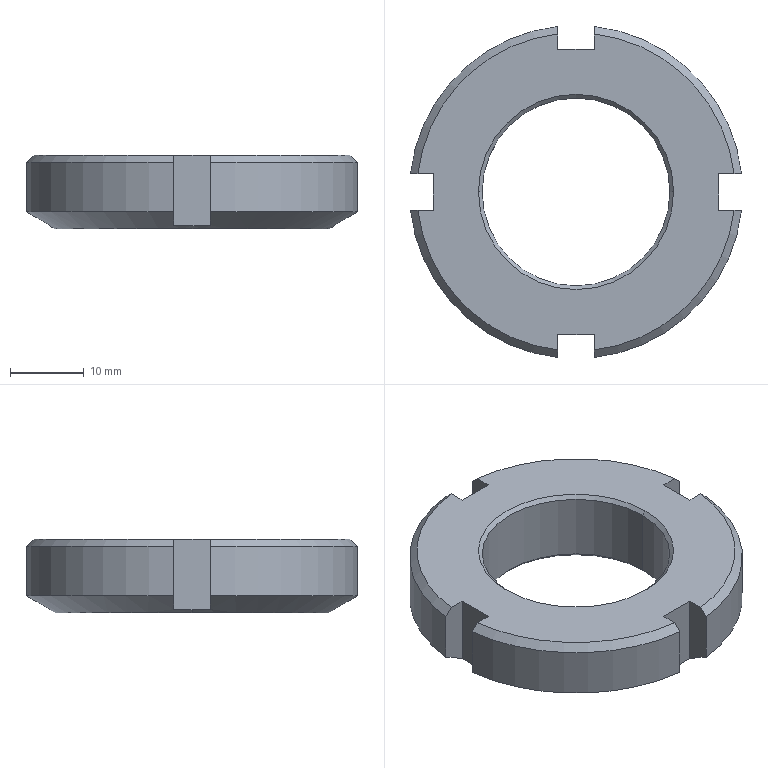Part | SolidWorks | features Chamfer 3, CirPattern 1, Cut 1, Extrusion 1 | 1 solid | 30 faces | box 44.721 x 44.721 x 10 mm | volume 9603 mm3 | plane 14 | cone 10 | cylinder 6 | commonest cylinder face diameters 45 x4 25.376 x2
STEP:
#1=CARTESIAN_POINT('',(-12.688,0.,9.5));
#2=VERTEX_POINT('',#1);
#3=CARTESIAN_POINT('',(12.688,0.,9.5));
#4=VERTEX_POINT('',#3);
#5=CARTESIAN_POINT('',(0.,0.,9.5));
#6=DIRECTION('',(0.,0.,1.));
#7=DIRECTION('',(1.,0.,0.));
#8=AXIS2_PLACEMENT_3D('',#5,#6,#7);
#9=CIRCLE('',#8,12.688);
#10=EDGE_CURVE('',#2,#4,#9,.T.);
#11=ORIENTED_EDGE('',*,*,#10,.F.);
#12=CARTESIAN_POINT('',(-13.188,0.,10.));
#13=VERTEX_POINT('',#12);
#14=CARTESIAN_POINT('',(-12.688,0.,9.5));
#15=DIRECTION('',(-0.7071,0.,0.7071));
#16=VECTOR('',#15,1000.);
#17=LINE('',#14,#16);
#18=EDGE_CURVE('',#2,#13,#17,.T.);
#19=ORIENTED_EDGE('',*,*,#18,.T.);
#20=CARTESIAN_POINT('',(13.188,0.,10.));
#21=VERTEX_POINT('',#20);
#22=CARTESIAN_POINT('',(0.,0.,10.));
#23=DIRECTION('',(0.,0.,-1.));
#24=DIRECTION('',(1.,0.,0.));
#25=AXIS2_PLACEMENT_3D('',#22,#23,#24);
#26=CIRCLE('',#25,13.188);
#27=EDGE_CURVE('',#21,#13,#26,.T.);
#28=ORIENTED_EDGE('',*,*,#27,.F.);
#29=CARTESIAN_POINT('',(12.688,0.,9.5));
#30=DIRECTION('',(0.7071,0.,0.7071));
#31=VECTOR('',#30,1000.);
#32=LINE('',#29,#31);
#33=EDGE_CURVE('',#4,#21,#32,.T.);
#34=ORIENTED_EDGE('',*,*,#33,.F.);
#35=EDGE_LOOP('',(#11,#19,#28,#34));
#36=FACE_OUTER_BOUND('',#35,.T.);
#37=CARTESIAN_POINT('',(0.,0.,9.5));
#38=DIRECTION('',(0.,0.,1.));
#39=DIRECTION('',(1.,0.,0.));
#40=AXIS2_PLACEMENT_3D('',#37,#38,#39);
#41=CONICAL_SURFACE('',#40,12.688,0.7854);
#42=ADVANCED_FACE('',(#36),#41,.F.);
#43=CARTESIAN_POINT('',(12.688,0.,0.5));
#44=VERTEX_POINT('',#43);
#45=CARTESIAN_POINT('',(-12.688,0.,0.5));
#46=VERTEX_POINT('',#45);
#47=CARTESIAN_POINT('',(0.,0.,0.5));
#48=DIRECTION('',(0.,0.,-1.));
#49=DIRECTION('',(1.,0.,0.));
#50=AXIS2_PLACEMENT_3D('',#47,#48,#49);
#51=CIRCLE('',#50,12.688);
#52=EDGE_CURVE('',#44,#46,#51,.T.);
#53=ORIENTED_EDGE('',*,*,#52,.F.);
#54=CARTESIAN_POINT('',(13.188,0.,0.));
#55=VERTEX_POINT('',#54);
#56=CARTESIAN_POINT('',(13.188,0.,0.));
#57=DIRECTION('',(0.7071,0.,-0.7071));
#58=VECTOR('',#57,1000.);
#59=LINE('',#56,#58);
#60=EDGE_CURVE('',#44,#55,#59,.T.);
#61=ORIENTED_EDGE('',*,*,#60,.T.);
#62=CARTESIAN_POINT('',(-13.188,0.,0.));
#63=VERTEX_POINT('',#62);
#64=CARTESIAN_POINT('',(0.,0.,0.));
#65=DIRECTION('',(0.,0.,1.));
#66=DIRECTION('',(1.,0.,0.));
#67=AXIS2_PLACEMENT_3D('',#64,#65,#66);
#68=CIRCLE('',#67,13.188);
#69=EDGE_CURVE('',#63,#55,#68,.T.);
#70=ORIENTED_EDGE('',*,*,#69,.F.);
#71=CARTESIAN_POINT('',(-13.188,0.,0.));
#72=DIRECTION('',(-0.7071,0.,-0.7071));
#73=VECTOR('',#72,1000.);
#74=LINE('',#71,#73);
#75=EDGE_CURVE('',#46,#63,#74,.T.);
#76=ORIENTED_EDGE('',*,*,#75,.F.);
#77=EDGE_LOOP('',(#53,#61,#70,#76));
#78=FACE_OUTER_BOUND('',#77,.T.);
#79=CARTESIAN_POINT('',(0.,0.,0.));
#80=DIRECTION('',(0.,0.,-1.));
#81=DIRECTION('',(-1.,0.,0.));
#82=AXIS2_PLACEMENT_3D('',#79,#80,#81);
#83=CONICAL_SURFACE('',#82,13.188,0.7854);
#84=ADVANCED_FACE('',(#78),#83,.F.);
#85=CARTESIAN_POINT('',(-18.5,0.,0.));
#86=VERTEX_POINT('',#85);
#87=CARTESIAN_POINT('',(18.5,0.,0.));
#88=VERTEX_POINT('',#87);
#89=CARTESIAN_POINT('',(0.,0.,0.));
#90=DIRECTION('',(0.,0.,-1.));
#91=DIRECTION('',(1.,0.,0.));
#92=AXIS2_PLACEMENT_3D('',#89,#90,#91);
#93=CIRCLE('',#92,18.5);
#94=EDGE_CURVE('',#86,#88,#93,.T.);
#95=ORIENTED_EDGE('',*,*,#94,.F.);
#96=CARTESIAN_POINT('',(-19.261,0.,0.4392));
#97=VERTEX_POINT('',#96);
#98=CARTESIAN_POINT('',(-22.5,0.,2.309));
#99=DIRECTION('',(-0.866,0.,0.5));
#100=VECTOR('',#99,1000.);
#101=LINE('',#98,#100);
#102=EDGE_CURVE('',#86,#97,#101,.T.);
#103=ORIENTED_EDGE('',*,*,#102,.T.);
#104=CARTESIAN_POINT('',(-19.261,2.5,0.5325));
#105=VERTEX_POINT('',#104);
#106=CARTESIAN_POINT('',(-19.261,2.5,0.5325));
#107=CARTESIAN_POINT('',(-19.261,1.67,0.4708));
#108=CARTESIAN_POINT('',(-19.261,0.8366,0.4392));
#109=CARTESIAN_POINT('',(-19.261,0.,0.4392));
#110=B_SPLINE_CURVE_WITH_KNOTS('',3,(#106,#107,#108,#109),.UNSPECIFIED.,.F.,.F.,(4,4),(0.006772,0.009268),.UNSPECIFIED.);
#111=EDGE_CURVE('',#105,#97,#110,.T.);
#112=ORIENTED_EDGE('',*,*,#111,.F.);
#113=CARTESIAN_POINT('',(-22.361,2.5,2.309));
#114=VERTEX_POINT('',#113);
#115=CARTESIAN_POINT('',(-22.361,2.5,2.309));
#116=CARTESIAN_POINT('',(-21.328,2.5,1.717));
#117=CARTESIAN_POINT('',(-20.294,2.5,1.124));
#118=CARTESIAN_POINT('',(-19.261,2.5,0.5325));
#119=B_SPLINE_CURVE_WITH_KNOTS('',3,(#115,#116,#117,#118),.UNSPECIFIED.,.F.,.F.,(4,4),(0.00673,0.0103),.UNSPECIFIED.);
#120=EDGE_CURVE('',#114,#105,#119,.T.);
#121=ORIENTED_EDGE('',*,*,#120,.F.);
#122=CARTESIAN_POINT('',(-2.5,22.361,2.309));
#123=VERTEX_POINT('',#122);
#124=CARTESIAN_POINT('',(0.,0.,2.309));
#125=DIRECTION('',(0.,0.,1.));
#126=DIRECTION('',(1.,0.,0.));
#127=AXIS2_PLACEMENT_3D('',#124,#125,#126);
#128=CIRCLE('',#127,22.5);
#129=EDGE_CURVE('',#123,#114,#128,.T.);
#130=ORIENTED_EDGE('',*,*,#129,.F.);
#131=CARTESIAN_POINT('',(-2.5,19.261,0.5325));
#132=VERTEX_POINT('',#131);
#133=CARTESIAN_POINT('',(-2.5,19.261,0.5325));
#134=CARTESIAN_POINT('',(-2.5,20.294,1.124));
#135=CARTESIAN_POINT('',(-2.5,21.328,1.717));
#136=CARTESIAN_POINT('',(-2.5,22.361,2.309));
#137=B_SPLINE_CURVE_WITH_KNOTS('',3,(#133,#134,#135,#136),.UNSPECIFIED.,.F.,.F.,(4,4),(0.006995,0.01057),.UNSPECIFIED.);
#138=EDGE_CURVE('',#132,#123,#137,.T.);
#139=ORIENTED_EDGE('',*,*,#138,.F.);
#140=CARTESIAN_POINT('',(2.5,19.261,0.5325));
#141=VERTEX_POINT('',#140);
#142=CARTESIAN_POINT('',(2.5,19.261,0.5325));
#143=CARTESIAN_POINT('',(1.673,19.261,0.471));
#144=CARTESIAN_POINT('',(0.8424,19.261,0.4394));
#145=CARTESIAN_POINT('',(-0.8248,19.261,0.439));
#146=CARTESIAN_POINT('',(-1.665,19.261,0.4704));
#147=CARTESIAN_POINT('',(-2.5,19.261,0.5325));
#148=B_SPLINE_CURVE_WITH_KNOTS('',3,(#142,#143,#144,#145,#146,#147),.UNSPECIFIED.,.F.,.F.,(4,2,4),(0.006772,0.009259,0.01175),.UNSPECIFIED.);
#149=EDGE_CURVE('',#141,#132,#148,.T.);
#150=ORIENTED_EDGE('',*,*,#149,.F.);
#151=CARTESIAN_POINT('',(2.5,22.361,2.309));
#152=VERTEX_POINT('',#151);
#153=CARTESIAN_POINT('',(2.5,22.361,2.309));
#154=CARTESIAN_POINT('',(2.5,21.328,1.717));
#155=CARTESIAN_POINT('',(2.5,20.294,1.124));
#156=CARTESIAN_POINT('',(2.5,19.261,0.5325));
#157=B_SPLINE_CURVE_WITH_KNOTS('',3,(#153,#154,#155,#156),.UNSPECIFIED.,.F.,.F.,(4,4),(0.004139,0.007712),.UNSPECIFIED.);
#158=EDGE_CURVE('',#152,#141,#157,.T.);
#159=ORIENTED_EDGE('',*,*,#158,.F.);
#160=CARTESIAN_POINT('',(22.361,2.5,2.309));
#161=VERTEX_POINT('',#160);
#162=CARTESIAN_POINT('',(0.,0.,2.309));
#163=DIRECTION('',(0.,0.,1.));
#164=DIRECTION('',(1.,0.,0.));
#165=AXIS2_PLACEMENT_3D('',#162,#163,#164);
#166=CIRCLE('',#165,22.5);
#167=EDGE_CURVE('',#161,#152,#166,.T.);
#168=ORIENTED_EDGE('',*,*,#167,.F.);
#169=CARTESIAN_POINT('',(19.261,2.5,0.5325));
#170=VERTEX_POINT('',#169);
#171=CARTESIAN_POINT('',(19.261,2.5,0.5325));
#172=CARTESIAN_POINT('',(20.294,2.5,1.124));
#173=CARTESIAN_POINT('',(21.328,2.5,1.717));
#174=CARTESIAN_POINT('',(22.361,2.5,2.309));
#175=B_SPLINE_CURVE_WITH_KNOTS('',3,(#171,#172,#173,#174),.UNSPECIFIED.,.F.,.F.,(4,4),(0.006995,0.01057),.UNSPECIFIED.);
#176=EDGE_CURVE('',#170,#161,#175,.T.);
#177=ORIENTED_EDGE('',*,*,#176,.F.);
#178=CARTESIAN_POINT('',(19.261,0.,0.4392));
#179=VERTEX_POINT('',#178);
#180=CARTESIAN_POINT('',(19.261,0.,0.4392));
#181=CARTESIAN_POINT('',(19.261,0.8366,0.4392));
#182=CARTESIAN_POINT('',(19.261,1.67,0.4708));
#183=CARTESIAN_POINT('',(19.261,2.5,0.5325));
#184=B_SPLINE_CURVE_WITH_KNOTS('',3,(#180,#181,#182,#183),.UNSPECIFIED.,.F.,.F.,(4,4),(0.01297,0.01547),.UNSPECIFIED.);
#185=EDGE_CURVE('',#179,#170,#184,.T.);
#186=ORIENTED_EDGE('',*,*,#185,.F.);
#187=CARTESIAN_POINT('',(22.5,0.,2.309));
#188=DIRECTION('',(0.866,0.,0.5));
#189=VECTOR('',#188,1000.);
#190=LINE('',#187,#189);
#191=EDGE_CURVE('',#88,#179,#190,.T.);
#192=ORIENTED_EDGE('',*,*,#191,.F.);
#193=EDGE_LOOP('',(#95,#103,#112,#121,#130,#139,#150,#159,#168,#177,#186,#192));
#194=FACE_OUTER_BOUND('',#193,.T.);
#195=CARTESIAN_POINT('',(0.,0.,2.309));
#196=DIRECTION('',(0.,0.,1.));
#197=DIRECTION('',(1.,0.,0.));
#198=AXIS2_PLACEMENT_3D('',#195,#196,#197);
#199=CONICAL_SURFACE('',#198,22.5,1.047);
#200=ADVANCED_FACE('',(#194),#199,.T.);
#201=ORIENTED_EDGE('',*,*,#10,.T.);
#202=CARTESIAN_POINT('',(12.688,0.,10.));
#203=DIRECTION('',(0.,0.,-1.));
#204=VECTOR('',#203,1000.);
#205=LINE('',#202,#204);
#206=EDGE_CURVE('',#4,#44,#205,.T.);
#207=ORIENTED_EDGE('',*,*,#206,.T.);
#208=ORIENTED_EDGE('',*,*,#52,.T.);
#209=CARTESIAN_POINT('',(-12.688,0.,10.));
#210=DIRECTION('',(0.,0.,-1.));
#211=VECTOR('',#210,1000.);
#212=LINE('',#209,#211);
#213=EDGE_CURVE('',#2,#46,#212,.T.);
#214=ORIENTED_EDGE('',*,*,#213,.F.);
#215=EDGE_LOOP('',(#201,#207,#208,#214));
#216=FACE_OUTER_BOUND('',#215,.T.);
#217=CARTESIAN_POINT('',(0.,0.,10.));
#218=DIRECTION('',(0.,0.,-1.));
#219=DIRECTION('',(-1.,0.,0.));
#220=AXIS2_PLACEMENT_3D('',#217,#218,#219);
#221=CYLINDRICAL_SURFACE('',#220,12.688);
#222=ADVANCED_FACE('',(#216),#221,.F.);
#223=CARTESIAN_POINT('',(2.5,22.361,9.));
#224=VERTEX_POINT('',#223);
#225=CARTESIAN_POINT('',(22.361,2.5,9.));
#226=VERTEX_POINT('',#225);
#227=CARTESIAN_POINT('',(0.,0.,9.));
#228=DIRECTION('',(0.,0.,-1.));
#229=DIRECTION('',(1.,0.,0.));
#230=AXIS2_PLACEMENT_3D('',#227,#228,#229);
#231=CIRCLE('',#230,22.5);
#232=EDGE_CURVE('',#224,#226,#231,.T.);
#233=ORIENTED_EDGE('',*,*,#232,.T.);
#234=CARTESIAN_POINT('',(22.361,2.5,0.));
#235=DIRECTION('',(0.,0.,1.));
#236=VECTOR('',#235,1000.);
#237=LINE('',#234,#236);
#238=EDGE_CURVE('',#161,#226,#237,.T.);
#239=ORIENTED_EDGE('',*,*,#238,.F.);
#240=ORIENTED_EDGE('',*,*,#167,.T.);
#241=CARTESIAN_POINT('',(2.5,22.361,0.));
#242=DIRECTION('',(0.,0.,1.));
#243=VECTOR('',#242,1000.);
#244=LINE('',#241,#243);
#245=EDGE_CURVE('',#152,#224,#244,.T.);
#246=ORIENTED_EDGE('',*,*,#245,.T.);
#247=EDGE_LOOP('',(#233,#239,#240,#246));
#248=FACE_OUTER_BOUND('',#247,.T.);
#249=CARTESIAN_POINT('',(0.,0.,10.));
#250=DIRECTION('',(0.,0.,-1.));
#251=DIRECTION('',(-1.,0.,0.));
#252=AXIS2_PLACEMENT_3D('',#249,#250,#251);
#253=CYLINDRICAL_SURFACE('',#252,22.5);
#254=ADVANCED_FACE('',(#248),#253,.T.);
#255=CARTESIAN_POINT('',(21.354,2.5,10.));
#256=VERTEX_POINT('',#255);
#257=CARTESIAN_POINT('',(22.361,2.5,9.));
#258=CARTESIAN_POINT('',(22.082,2.5,9.277));
#259=CARTESIAN_POINT('',(21.804,2.5,9.553));
#260=CARTESIAN_POINT('',(21.526,2.5,9.83));
#261=CARTESIAN_POINT('',(21.468,2.5,9.886));
#262=CARTESIAN_POINT('',(21.411,2.5,9.943));
#263=CARTESIAN_POINT('',(21.354,2.5,10.));
#264=B_SPLINE_CURVE_WITH_KNOTS('',3,(#257,#258,#259,#260,#261,#262,#263),.UNSPECIFIED.,.F.,.F.,(4,3,4),(0.005158,0.006335,0.006577),.UNSPECIFIED.);
#265=EDGE_CURVE('',#226,#256,#264,.T.);
#266=ORIENTED_EDGE('',*,*,#265,.F.);
#267=ORIENTED_EDGE('',*,*,#232,.F.);
#268=CARTESIAN_POINT('',(2.5,21.354,10.));
#269=VERTEX_POINT('',#268);
#270=CARTESIAN_POINT('',(2.5,21.354,10.));
#271=CARTESIAN_POINT('',(2.5,21.411,9.943));
#272=CARTESIAN_POINT('',(2.5,21.468,9.886));
#273=CARTESIAN_POINT('',(2.5,21.526,9.83));
#274=CARTESIAN_POINT('',(2.5,21.804,9.553));
#275=CARTESIAN_POINT('',(2.5,22.082,9.277));
#276=CARTESIAN_POINT('',(2.5,22.361,9.));
#277=B_SPLINE_CURVE_WITH_KNOTS('',3,(#270,#271,#272,#273,#274,#275,#276),.UNSPECIFIED.,.F.,.F.,(4,3,4),(0.006094,0.006335,0.007513),.UNSPECIFIED.);
#278=EDGE_CURVE('',#269,#224,#277,.T.);
#279=ORIENTED_EDGE('',*,*,#278,.F.);
#280=CARTESIAN_POINT('',(0.,0.,10.));
#281=DIRECTION('',(0.,0.,1.));
#282=DIRECTION('',(1.,0.,0.));
#283=AXIS2_PLACEMENT_3D('',#280,#281,#282);
#284=CIRCLE('',#283,21.5);
#285=EDGE_CURVE('',#256,#269,#284,.T.);
#286=ORIENTED_EDGE('',*,*,#285,.F.);
#287=EDGE_LOOP('',(#266,#267,#279,#286));
#288=FACE_OUTER_BOUND('',#287,.T.);
#289=CARTESIAN_POINT('',(0.,0.,10.));
#290=DIRECTION('',(0.,0.,-1.));
#291=DIRECTION('',(-1.,0.,0.));
#292=AXIS2_PLACEMENT_3D('',#289,#290,#291);
#293=CONICAL_SURFACE('',#292,21.5,0.7854);
#294=ADVANCED_FACE('',(#288),#293,.T.);
#295=CARTESIAN_POINT('',(-22.361,2.5,9.));
#296=VERTEX_POINT('',#295);
#297=CARTESIAN_POINT('',(-2.5,22.361,9.));
#298=VERTEX_POINT('',#297);
#299=CARTESIAN_POINT('',(0.,0.,9.));
#300=DIRECTION('',(0.,0.,-1.));
#301=DIRECTION('',(1.,0.,0.));
#302=AXIS2_PLACEMENT_3D('',#299,#300,#301);
#303=CIRCLE('',#302,22.5);
#304=EDGE_CURVE('',#296,#298,#303,.T.);
#305=ORIENTED_EDGE('',*,*,#304,.T.);
#306=CARTESIAN_POINT('',(-2.5,22.361,0.));
#307=DIRECTION('',(0.,0.,1.));
#308=VECTOR('',#307,1000.);
#309=LINE('',#306,#308);
#310=EDGE_CURVE('',#123,#298,#309,.T.);
#311=ORIENTED_EDGE('',*,*,#310,.F.);
#312=ORIENTED_EDGE('',*,*,#129,.T.);
#313=CARTESIAN_POINT('',(-22.361,2.5,0.));
#314=DIRECTION('',(0.,0.,1.));
#315=VECTOR('',#314,1000.);
#316=LINE('',#313,#315);
#317=EDGE_CURVE('',#114,#296,#316,.T.);
#318=ORIENTED_EDGE('',*,*,#317,.T.);
#319=EDGE_LOOP('',(#305,#311,#312,#318));
#320=FACE_OUTER_BOUND('',#319,.T.);
#321=CARTESIAN_POINT('',(0.,0.,10.));
#322=DIRECTION('',(0.,0.,-1.));
#323=DIRECTION('',(-1.,0.,0.));
#324=AXIS2_PLACEMENT_3D('',#321,#322,#323);
#325=CYLINDRICAL_SURFACE('',#324,22.5);
#326=ADVANCED_FACE('',(#320),#325,.T.);
#327=CARTESIAN_POINT('',(-2.5,21.354,10.));
#328=VERTEX_POINT('',#327);
#329=CARTESIAN_POINT('',(-2.5,22.361,9.));
#330=CARTESIAN_POINT('',(-2.5,22.082,9.277));
#331=CARTESIAN_POINT('',(-2.5,21.804,9.553));
#332=CARTESIAN_POINT('',(-2.5,21.526,9.83));
#333=CARTESIAN_POINT('',(-2.5,21.468,9.886));
#334=CARTESIAN_POINT('',(-2.5,21.411,9.943));
#335=CARTESIAN_POINT('',(-2.5,21.354,10.));
#336=B_SPLINE_CURVE_WITH_KNOTS('',3,(#329,#330,#331,#332,#333,#334,#335),.UNSPECIFIED.,.F.,.F.,(4,3,4),(0.005158,0.006335,0.006577),.UNSPECIFIED.);
#337=EDGE_CURVE('',#298,#328,#336,.T.);
#338=ORIENTED_EDGE('',*,*,#337,.F.);
#339=ORIENTED_EDGE('',*,*,#304,.F.);
#340=CARTESIAN_POINT('',(-21.354,2.5,10.));
#341=VERTEX_POINT('',#340);
#342=CARTESIAN_POINT('',(-21.354,2.5,10.));
#343=CARTESIAN_POINT('',(-21.541,2.5,9.814));
#344=CARTESIAN_POINT('',(-21.729,2.5,9.628));
#345=CARTESIAN_POINT('',(-21.916,2.5,9.442));
#346=CARTESIAN_POINT('',(-22.064,2.5,9.295));
#347=CARTESIAN_POINT('',(-22.212,2.5,9.147));
#348=CARTESIAN_POINT('',(-22.361,2.5,9.));
#349=B_SPLINE_CURVE_WITH_KNOTS('',3,(#342,#343,#344,#345,#346,#347,#348),.UNSPECIFIED.,.F.,.F.,(4,3,4),(0.005544,0.006335,0.006963),.UNSPECIFIED.);
#350=EDGE_CURVE('',#341,#296,#349,.T.);
#351=ORIENTED_EDGE('',*,*,#350,.F.);
#352=CARTESIAN_POINT('',(0.,0.,10.));
#353=DIRECTION('',(0.,0.,1.));
#354=DIRECTION('',(1.,0.,0.));
#355=AXIS2_PLACEMENT_3D('',#352,#353,#354);
#356=CIRCLE('',#355,21.5);
#357=EDGE_CURVE('',#328,#341,#356,.T.);
#358=ORIENTED_EDGE('',*,*,#357,.F.);
#359=EDGE_LOOP('',(#338,#339,#351,#358));
#360=FACE_OUTER_BOUND('',#359,.T.);
#361=CARTESIAN_POINT('',(0.,0.,10.));
#362=DIRECTION('',(0.,0.,-1.));
#363=DIRECTION('',(-1.,0.,0.));
#364=AXIS2_PLACEMENT_3D('',#361,#362,#363);
#365=CONICAL_SURFACE('',#364,21.5,0.7854);
#366=ADVANCED_FACE('',(#360),#365,.T.);
#367=CARTESIAN_POINT('',(-2.5,-22.361,9.));
#368=VERTEX_POINT('',#367);
#369=CARTESIAN_POINT('',(-22.361,-2.5,9.));
#370=VERTEX_POINT('',#369);
#371=CARTESIAN_POINT('',(0.,0.,9.));
#372=DIRECTION('',(0.,0.,-1.));
#373=DIRECTION('',(1.,0.,0.));
#374=AXIS2_PLACEMENT_3D('',#371,#372,#373);
#375=CIRCLE('',#374,22.5);
#376=EDGE_CURVE('',#368,#370,#375,.T.);
#377=ORIENTED_EDGE('',*,*,#376,.T.);
#378=CARTESIAN_POINT('',(-22.361,-2.5,2.309));
#379=VERTEX_POINT('',#378);
#380=CARTESIAN_POINT('',(-22.361,-2.5,0.));
#381=DIRECTION('',(0.,0.,1.));
#382=VECTOR('',#381,1000.);
#383=LINE('',#380,#382);
#384=EDGE_CURVE('',#379,#370,#383,.T.);
#385=ORIENTED_EDGE('',*,*,#384,.F.);
#386=CARTESIAN_POINT('',(-2.5,-22.361,2.309));
#387=VERTEX_POINT('',#386);
#388=CARTESIAN_POINT('',(0.,0.,2.309));
#389=DIRECTION('',(0.,0.,1.));
#390=DIRECTION('',(1.,0.,0.));
#391=AXIS2_PLACEMENT_3D('',#388,#389,#390);
#392=CIRCLE('',#391,22.5);
#393=EDGE_CURVE('',#379,#387,#392,.T.);
#394=ORIENTED_EDGE('',*,*,#393,.T.);
#395=CARTESIAN_POINT('',(-2.5,-22.361,0.));
#396=DIRECTION('',(0.,0.,1.));
#397=VECTOR('',#396,1000.);
#398=LINE('',#395,#397);
#399=EDGE_CURVE('',#387,#368,#398,.T.);
#400=ORIENTED_EDGE('',*,*,#399,.T.);
#401=EDGE_LOOP('',(#377,#385,#394,#400));
#402=FACE_OUTER_BOUND('',#401,.T.);
#403=CARTESIAN_POINT('',(0.,0.,10.));
#404=DIRECTION('',(0.,0.,-1.));
#405=DIRECTION('',(-1.,0.,0.));
#406=AXIS2_PLACEMENT_3D('',#403,#404,#405);
#407=CYLINDRICAL_SURFACE('',#406,22.5);
#408=ADVANCED_FACE('',(#402),#407,.T.);
#409=CARTESIAN_POINT('',(-21.354,-2.5,10.));
#410=VERTEX_POINT('',#409);
#411=CARTESIAN_POINT('',(-22.361,-2.5,9.));
#412=CARTESIAN_POINT('',(-22.212,-2.5,9.147));
#413=CARTESIAN_POINT('',(-22.064,-2.5,9.295));
#414=CARTESIAN_POINT('',(-21.916,-2.5,9.442));
#415=CARTESIAN_POINT('',(-21.729,-2.5,9.628));
#416=CARTESIAN_POINT('',(-21.541,-2.5,9.814));
#417=CARTESIAN_POINT('',(-21.354,-2.5,10.));
#418=B_SPLINE_CURVE_WITH_KNOTS('',3,(#411,#412,#413,#414,#415,#416,#417),.UNSPECIFIED.,.F.,.F.,(4,3,4),(0.005708,0.006335,0.007127),.UNSPECIFIED.);
#419=EDGE_CURVE('',#370,#410,#418,.T.);
#420=ORIENTED_EDGE('',*,*,#419,.F.);
#421=ORIENTED_EDGE('',*,*,#376,.F.);
#422=CARTESIAN_POINT('',(-2.5,-21.354,10.));
#423=VERTEX_POINT('',#422);
#424=CARTESIAN_POINT('',(-2.5,-21.354,10.));
#425=CARTESIAN_POINT('',(-2.5,-21.541,9.814));
#426=CARTESIAN_POINT('',(-2.5,-21.729,9.628));
#427=CARTESIAN_POINT('',(-2.5,-21.916,9.442));
#428=CARTESIAN_POINT('',(-2.5,-22.064,9.295));
#429=CARTESIAN_POINT('',(-2.5,-22.212,9.147));
#430=CARTESIAN_POINT('',(-2.5,-22.361,9.));
#431=B_SPLINE_CURVE_WITH_KNOTS('',3,(#424,#425,#426,#427,#428,#429,#430),.UNSPECIFIED.,.F.,.F.,(4,3,4),(0.005544,0.006335,0.006963),.UNSPECIFIED.);
#432=EDGE_CURVE('',#423,#368,#431,.T.);
#433=ORIENTED_EDGE('',*,*,#432,.F.);
#434=CARTESIAN_POINT('',(0.,0.,10.));
#435=DIRECTION('',(0.,0.,1.));
#436=DIRECTION('',(1.,0.,0.));
#437=AXIS2_PLACEMENT_3D('',#434,#435,#436);
#438=CIRCLE('',#437,21.5);
#439=EDGE_CURVE('',#410,#423,#438,.T.);
#440=ORIENTED_EDGE('',*,*,#439,.F.);
#441=EDGE_LOOP('',(#420,#421,#433,#440));
#442=FACE_OUTER_BOUND('',#441,.T.);
#443=CARTESIAN_POINT('',(0.,0.,10.));
#444=DIRECTION('',(0.,0.,-1.));
#445=DIRECTION('',(-1.,0.,0.));
#446=AXIS2_PLACEMENT_3D('',#443,#444,#445);
#447=CONICAL_SURFACE('',#446,21.5,0.7854);
#448=ADVANCED_FACE('',(#442),#447,.T.);
#449=ORIENTED_EDGE('',*,*,#27,.T.);
#450=CARTESIAN_POINT('',(0.,0.,10.));
#451=DIRECTION('',(0.,0.,-1.));
#452=DIRECTION('',(1.,0.,0.));
#453=AXIS2_PLACEMENT_3D('',#450,#451,#452);
#454=CIRCLE('',#453,13.188);
#455=EDGE_CURVE('',#13,#21,#454,.T.);
#456=ORIENTED_EDGE('',*,*,#455,.T.);
#457=EDGE_LOOP('',(#449,#456));
#458=FACE_BOUND('',#457,.T.);
#459=CARTESIAN_POINT('',(19.261,2.5,10.));
#460=VERTEX_POINT('',#459);
#461=CARTESIAN_POINT('',(19.261,2.5,10.));
#462=DIRECTION('',(-1.,0.,0.));
#463=VECTOR('',#462,1000.);
#464=LINE('',#461,#463);
#465=EDGE_CURVE('',#256,#460,#464,.T.);
#466=ORIENTED_EDGE('',*,*,#465,.F.);
#467=ORIENTED_EDGE('',*,*,#285,.T.);
#468=CARTESIAN_POINT('',(2.5,19.261,10.));
#469=VERTEX_POINT('',#468);
#470=CARTESIAN_POINT('',(2.5,19.261,10.));
#471=DIRECTION('',(0.,1.,0.));
#472=VECTOR('',#471,1000.);
#473=LINE('',#470,#472);
#474=EDGE_CURVE('',#469,#269,#473,.T.);
#475=ORIENTED_EDGE('',*,*,#474,.F.);
#476=CARTESIAN_POINT('',(-2.5,19.261,10.));
#477=VERTEX_POINT('',#476);
#478=CARTESIAN_POINT('',(2.5,19.261,10.));
#479=DIRECTION('',(1.,0.,0.));
#480=VECTOR('',#479,1000.);
#481=LINE('',#478,#480);
#482=EDGE_CURVE('',#477,#469,#481,.T.);
#483=ORIENTED_EDGE('',*,*,#482,.F.);
#484=CARTESIAN_POINT('',(-2.5,19.261,10.));
#485=DIRECTION('',(0.,-1.,0.));
#486=VECTOR('',#485,1000.);
#487=LINE('',#484,#486);
#488=EDGE_CURVE('',#328,#477,#487,.T.);
#489=ORIENTED_EDGE('',*,*,#488,.F.);
#490=ORIENTED_EDGE('',*,*,#357,.T.);
#491=CARTESIAN_POINT('',(-19.261,2.5,10.));
#492=VERTEX_POINT('',#491);
#493=CARTESIAN_POINT('',(-19.261,2.5,10.));
#494=DIRECTION('',(-1.,0.,0.));
#495=VECTOR('',#494,1000.);
#496=LINE('',#493,#495);
#497=EDGE_CURVE('',#492,#341,#496,.T.);
#498=ORIENTED_EDGE('',*,*,#497,.F.);
#499=CARTESIAN_POINT('',(-19.261,-2.5,10.));
#500=VERTEX_POINT('',#499);
#501=CARTESIAN_POINT('',(-19.261,2.5,10.));
#502=DIRECTION('',(0.,1.,0.));
#503=VECTOR('',#502,1000.);
#504=LINE('',#501,#503);
#505=EDGE_CURVE('',#500,#492,#504,.T.);
#506=ORIENTED_EDGE('',*,*,#505,.F.);
#507=CARTESIAN_POINT('',(-19.261,-2.5,10.));
#508=DIRECTION('',(1.,0.,0.));
#509=VECTOR('',#508,1000.);
#510=LINE('',#507,#509);
#511=EDGE_CURVE('',#410,#500,#510,.T.);
#512=ORIENTED_EDGE('',*,*,#511,.F.);
#513=ORIENTED_EDGE('',*,*,#439,.T.);
#514=CARTESIAN_POINT('',(-2.5,-19.261,10.));
#515=VERTEX_POINT('',#514);
#516=CARTESIAN_POINT('',(-2.5,-19.261,10.));
#517=DIRECTION('',(0.,-1.,0.));
#518=VECTOR('',#517,1000.);
#519=LINE('',#516,#518);
#520=EDGE_CURVE('',#515,#423,#519,.T.);
#521=ORIENTED_EDGE('',*,*,#520,.F.);
#522=CARTESIAN_POINT('',(2.5,-19.261,10.));
#523=VERTEX_POINT('',#522);
#524=CARTESIAN_POINT('',(-2.5,-19.261,10.));
#525=DIRECTION('',(-1.,0.,0.));
#526=VECTOR('',#525,1000.);
#527=LINE('',#524,#526);
#528=EDGE_CURVE('',#523,#515,#527,.T.);
#529=ORIENTED_EDGE('',*,*,#528,.F.);
#530=CARTESIAN_POINT('',(2.5,-21.354,10.));
#531=VERTEX_POINT('',#530);
#532=CARTESIAN_POINT('',(2.5,-19.261,10.));
#533=DIRECTION('',(0.,1.,0.));
#534=VECTOR('',#533,1000.);
#535=LINE('',#532,#534);
#536=EDGE_CURVE('',#531,#523,#535,.T.);
#537=ORIENTED_EDGE('',*,*,#536,.F.);
#538=CARTESIAN_POINT('',(21.354,-2.5,10.));
#539=VERTEX_POINT('',#538);
#540=CARTESIAN_POINT('',(0.,0.,10.));
#541=DIRECTION('',(0.,0.,1.));
#542=DIRECTION('',(1.,0.,0.));
#543=AXIS2_PLACEMENT_3D('',#540,#541,#542);
#544=CIRCLE('',#543,21.5);
#545=EDGE_CURVE('',#531,#539,#544,.T.);
#546=ORIENTED_EDGE('',*,*,#545,.T.);
#547=CARTESIAN_POINT('',(19.261,-2.5,10.));
#548=VERTEX_POINT('',#547);
#549=CARTESIAN_POINT('',(19.261,-2.5,10.));
#550=DIRECTION('',(1.,0.,0.));
#551=VECTOR('',#550,1000.);
#552=LINE('',#549,#551);
#553=EDGE_CURVE('',#548,#539,#552,.T.);
#554=ORIENTED_EDGE('',*,*,#553,.F.);
#555=CARTESIAN_POINT('',(19.261,-2.5,10.));
#556=DIRECTION('',(0.,-1.,0.));
#557=VECTOR('',#556,1000.);
#558=LINE('',#555,#557);
#559=EDGE_CURVE('',#460,#548,#558,.T.);
#560=ORIENTED_EDGE('',*,*,#559,.F.);
#561=EDGE_LOOP('',(#466,#467,#475,#483,#489,#490,#498,#506,#512,#513,#521,#529,#537,#546,#554,#560));
#562=FACE_OUTER_BOUND('',#561,.T.);
#563=CARTESIAN_POINT('',(0.,0.,10.));
#564=DIRECTION('',(0.,0.,1.));
#565=DIRECTION('',(1.,0.,0.));
#566=AXIS2_PLACEMENT_3D('',#563,#564,#565);
#567=PLANE('',#566);
#568=ADVANCED_FACE('',(#458,#562),#567,.T.);
#569=ORIENTED_EDGE('',*,*,#69,.T.);
#570=CARTESIAN_POINT('',(0.,0.,0.));
#571=DIRECTION('',(0.,0.,1.));
#572=DIRECTION('',(1.,0.,0.));
#573=AXIS2_PLACEMENT_3D('',#570,#571,#572);
#574=CIRCLE('',#573,13.188);
#575=EDGE_CURVE('',#55,#63,#574,.T.);
#576=ORIENTED_EDGE('',*,*,#575,.T.);
#577=EDGE_LOOP('',(#569,#576));
#578=FACE_BOUND('',#577,.T.);
#579=CARTESIAN_POINT('',(0.,0.,0.));
#580=DIRECTION('',(0.,0.,-1.));
#581=DIRECTION('',(1.,0.,0.));
#582=AXIS2_PLACEMENT_3D('',#579,#580,#581);
#583=CIRCLE('',#582,18.5);
#584=EDGE_CURVE('',#88,#86,#583,.T.);
#585=ORIENTED_EDGE('',*,*,#584,.T.);
#586=ORIENTED_EDGE('',*,*,#94,.T.);
#587=EDGE_LOOP('',(#585,#586));
#588=FACE_OUTER_BOUND('',#587,.T.);
#589=CARTESIAN_POINT('',(0.,0.,0.));
#590=DIRECTION('',(0.,0.,1.));
#591=DIRECTION('',(1.,0.,0.));
#592=AXIS2_PLACEMENT_3D('',#589,#590,#591);
#593=PLANE('',#592);
#594=ADVANCED_FACE('',(#578,#588),#593,.F.);
#595=CARTESIAN_POINT('',(2.5,-22.361,2.309));
#596=VERTEX_POINT('',#595);
#597=CARTESIAN_POINT('',(22.361,-2.5,2.309));
#598=VERTEX_POINT('',#597);
#599=CARTESIAN_POINT('',(0.,0.,2.309));
#600=DIRECTION('',(0.,0.,1.));
#601=DIRECTION('',(1.,0.,0.));
#602=AXIS2_PLACEMENT_3D('',#599,#600,#601);
#603=CIRCLE('',#602,22.5);
#604=EDGE_CURVE('',#596,#598,#603,.T.);
#605=ORIENTED_EDGE('',*,*,#604,.T.);
#606=CARTESIAN_POINT('',(22.361,-2.5,9.));
#607=VERTEX_POINT('',#606);
#608=CARTESIAN_POINT('',(22.361,-2.5,0.));
#609=DIRECTION('',(0.,0.,1.));
#610=VECTOR('',#609,1000.);
#611=LINE('',#608,#610);
#612=EDGE_CURVE('',#598,#607,#611,.T.);
#613=ORIENTED_EDGE('',*,*,#612,.T.);
#614=CARTESIAN_POINT('',(2.5,-22.361,9.));
#615=VERTEX_POINT('',#614);
#616=CARTESIAN_POINT('',(0.,0.,9.));
#617=DIRECTION('',(0.,0.,-1.));
#618=DIRECTION('',(1.,0.,0.));
#619=AXIS2_PLACEMENT_3D('',#616,#617,#618);
#620=CIRCLE('',#619,22.5);
#621=EDGE_CURVE('',#607,#615,#620,.T.);
#622=ORIENTED_EDGE('',*,*,#621,.T.);
#623=CARTESIAN_POINT('',(2.5,-22.361,0.));
#624=DIRECTION('',(0.,0.,1.));
#625=VECTOR('',#624,1000.);
#626=LINE('',#623,#625);
#627=EDGE_CURVE('',#596,#615,#626,.T.);
#628=ORIENTED_EDGE('',*,*,#627,.F.);
#629=EDGE_LOOP('',(#605,#613,#622,#628));
#630=FACE_OUTER_BOUND('',#629,.T.);
#631=CARTESIAN_POINT('',(0.,0.,10.));
#632=DIRECTION('',(0.,0.,-1.));
#633=DIRECTION('',(-1.,0.,0.));
#634=AXIS2_PLACEMENT_3D('',#631,#632,#633);
#635=CYLINDRICAL_SURFACE('',#634,22.5);
#636=ADVANCED_FACE('',(#630),#635,.T.);
#637=ORIENTED_EDGE('',*,*,#206,.F.);
#638=CARTESIAN_POINT('',(0.,0.,9.5));
#639=DIRECTION('',(0.,0.,1.));
#640=DIRECTION('',(1.,0.,0.));
#641=AXIS2_PLACEMENT_3D('',#638,#639,#640);
#642=CIRCLE('',#641,12.688);
#643=EDGE_CURVE('',#4,#2,#642,.T.);
#644=ORIENTED_EDGE('',*,*,#643,.T.);
#645=ORIENTED_EDGE('',*,*,#213,.T.);
#646=CARTESIAN_POINT('',(0.,0.,0.5));
#647=DIRECTION('',(0.,0.,-1.));
#648=DIRECTION('',(1.,0.,0.));
#649=AXIS2_PLACEMENT_3D('',#646,#647,#648);
#650=CIRCLE('',#649,12.688);
#651=EDGE_CURVE('',#46,#44,#650,.T.);
#652=ORIENTED_EDGE('',*,*,#651,.T.);
#653=EDGE_LOOP('',(#637,#644,#645,#652));
#654=FACE_OUTER_BOUND('',#653,.T.);
#655=CARTESIAN_POINT('',(0.,0.,10.));
#656=DIRECTION('',(0.,0.,-1.));
#657=DIRECTION('',(-1.,0.,0.));
#658=AXIS2_PLACEMENT_3D('',#655,#656,#657);
#659=CYLINDRICAL_SURFACE('',#658,12.688);
#660=ADVANCED_FACE('',(#654),#659,.F.);
#661=CARTESIAN_POINT('',(21.354,-2.5,10.));
#662=CARTESIAN_POINT('',(21.411,-2.5,9.943));
#663=CARTESIAN_POINT('',(21.468,-2.5,9.886));
#664=CARTESIAN_POINT('',(21.526,-2.5,9.83));
#665=CARTESIAN_POINT('',(21.804,-2.5,9.553));
#666=CARTESIAN_POINT('',(22.082,-2.5,9.277));
#667=CARTESIAN_POINT('',(22.361,-2.5,9.));
#668=B_SPLINE_CURVE_WITH_KNOTS('',3,(#661,#662,#663,#664,#665,#666,#667),.UNSPECIFIED.,.F.,.F.,(4,3,4),(0.006094,0.006335,0.007513),.UNSPECIFIED.);
#669=EDGE_CURVE('',#539,#607,#668,.T.);
#670=ORIENTED_EDGE('',*,*,#669,.F.);
#671=ORIENTED_EDGE('',*,*,#545,.F.);
#672=CARTESIAN_POINT('',(2.5,-22.361,9.));
#673=CARTESIAN_POINT('',(2.5,-22.212,9.147));
#674=CARTESIAN_POINT('',(2.5,-22.064,9.295));
#675=CARTESIAN_POINT('',(2.5,-21.916,9.442));
#676=CARTESIAN_POINT('',(2.5,-21.729,9.628));
#677=CARTESIAN_POINT('',(2.5,-21.541,9.814));
#678=CARTESIAN_POINT('',(2.5,-21.354,10.));
#679=B_SPLINE_CURVE_WITH_KNOTS('',3,(#672,#673,#674,#675,#676,#677,#678),.UNSPECIFIED.,.F.,.F.,(4,3,4),(0.005708,0.006335,0.007127),.UNSPECIFIED.);
#680=EDGE_CURVE('',#615,#531,#679,.T.);
#681=ORIENTED_EDGE('',*,*,#680,.F.);
#682=ORIENTED_EDGE('',*,*,#621,.F.);
#683=EDGE_LOOP('',(#670,#671,#681,#682));
#684=FACE_OUTER_BOUND('',#683,.T.);
#685=CARTESIAN_POINT('',(0.,0.,10.));
#686=DIRECTION('',(0.,0.,-1.));
#687=DIRECTION('',(-1.,0.,0.));
#688=AXIS2_PLACEMENT_3D('',#685,#686,#687);
#689=CONICAL_SURFACE('',#688,21.5,0.7854);
#690=ADVANCED_FACE('',(#684),#689,.T.);
#691=ORIENTED_EDGE('',*,*,#102,.F.);
#692=ORIENTED_EDGE('',*,*,#584,.F.);
#693=ORIENTED_EDGE('',*,*,#191,.T.);
#694=CARTESIAN_POINT('',(19.261,-2.5,0.5325));
#695=VERTEX_POINT('',#694);
#696=CARTESIAN_POINT('',(19.261,-2.5,0.5325));
#697=CARTESIAN_POINT('',(19.261,-1.667,0.4706));
#698=CARTESIAN_POINT('',(19.261,-0.8307,0.4392));
#699=CARTESIAN_POINT('',(19.261,0.,0.4392));
#700=B_SPLINE_CURVE_WITH_KNOTS('',3,(#696,#697,#698,#699),.UNSPECIFIED.,.F.,.F.,(4,4),(0.01048,0.01297),.UNSPECIFIED.);
#701=EDGE_CURVE('',#695,#179,#700,.T.);
#702=ORIENTED_EDGE('',*,*,#701,.F.);
#703=CARTESIAN_POINT('',(22.361,-2.5,2.309));
#704=CARTESIAN_POINT('',(21.328,-2.5,1.717));
#705=CARTESIAN_POINT('',(20.294,-2.5,1.124));
#706=CARTESIAN_POINT('',(19.261,-2.5,0.5325));
#707=B_SPLINE_CURVE_WITH_KNOTS('',3,(#703,#704,#705,#706),.UNSPECIFIED.,.F.,.F.,(4,4),(0.004139,0.007712),.UNSPECIFIED.);
#708=EDGE_CURVE('',#598,#695,#707,.T.);
#709=ORIENTED_EDGE('',*,*,#708,.F.);
#710=ORIENTED_EDGE('',*,*,#604,.F.);
#711=CARTESIAN_POINT('',(2.5,-19.261,0.5325));
#712=VERTEX_POINT('',#711);
#713=CARTESIAN_POINT('',(2.5,-19.261,0.5325));
#714=CARTESIAN_POINT('',(2.5,-20.294,1.124));
#715=CARTESIAN_POINT('',(2.5,-21.328,1.717));
#716=CARTESIAN_POINT('',(2.5,-22.361,2.309));
#717=B_SPLINE_CURVE_WITH_KNOTS('',3,(#713,#714,#715,#716),.UNSPECIFIED.,.F.,.F.,(4,4),(0.004404,0.007977),.UNSPECIFIED.);
#718=EDGE_CURVE('',#712,#596,#717,.T.);
#719=ORIENTED_EDGE('',*,*,#718,.F.);
#720=CARTESIAN_POINT('',(-2.5,-19.261,0.5325));
#721=VERTEX_POINT('',#720);
#722=CARTESIAN_POINT('',(-2.5,-19.261,0.5325));
#723=CARTESIAN_POINT('',(-1.665,-19.261,0.4704));
#724=CARTESIAN_POINT('',(-0.8248,-19.261,0.439));
#725=CARTESIAN_POINT('',(0.8424,-19.261,0.4394));
#726=CARTESIAN_POINT('',(1.673,-19.261,0.471));
#727=CARTESIAN_POINT('',(2.5,-19.261,0.5325));
#728=B_SPLINE_CURVE_WITH_KNOTS('',3,(#722,#723,#724,#725,#726,#727),.UNSPECIFIED.,.F.,.F.,(4,2,4),(0.01048,0.01298,0.01547),.UNSPECIFIED.);
#729=EDGE_CURVE('',#721,#712,#728,.T.);
#730=ORIENTED_EDGE('',*,*,#729,.F.);
#731=CARTESIAN_POINT('',(-2.5,-22.361,2.309));
#732=CARTESIAN_POINT('',(-2.5,-21.328,1.717));
#733=CARTESIAN_POINT('',(-2.5,-20.294,1.124));
#734=CARTESIAN_POINT('',(-2.5,-19.261,0.5325));
#735=B_SPLINE_CURVE_WITH_KNOTS('',3,(#731,#732,#733,#734),.UNSPECIFIED.,.F.,.F.,(4,4),(0.00673,0.0103),.UNSPECIFIED.);
#736=EDGE_CURVE('',#387,#721,#735,.T.);
#737=ORIENTED_EDGE('',*,*,#736,.F.);
#738=ORIENTED_EDGE('',*,*,#393,.F.);
#739=CARTESIAN_POINT('',(-19.261,-2.5,0.5325));
#740=VERTEX_POINT('',#739);
#741=CARTESIAN_POINT('',(-19.261,-2.5,0.5325));
#742=CARTESIAN_POINT('',(-20.294,-2.5,1.124));
#743=CARTESIAN_POINT('',(-21.328,-2.5,1.717));
#744=CARTESIAN_POINT('',(-22.361,-2.5,2.309));
#745=B_SPLINE_CURVE_WITH_KNOTS('',3,(#741,#742,#743,#744),.UNSPECIFIED.,.F.,.F.,(4,4),(0.004404,0.007977),.UNSPECIFIED.);
#746=EDGE_CURVE('',#740,#379,#745,.T.);
#747=ORIENTED_EDGE('',*,*,#746,.F.);
#748=CARTESIAN_POINT('',(-19.261,0.,0.4392));
#749=CARTESIAN_POINT('',(-19.261,-0.8307,0.4392));
#750=CARTESIAN_POINT('',(-19.261,-1.667,0.4706));
#751=CARTESIAN_POINT('',(-19.261,-2.5,0.5325));
#752=B_SPLINE_CURVE_WITH_KNOTS('',3,(#748,#749,#750,#751),.UNSPECIFIED.,.F.,.F.,(4,4),(0.009268,0.01175),.UNSPECIFIED.);
#753=EDGE_CURVE('',#97,#740,#752,.T.);
#754=ORIENTED_EDGE('',*,*,#753,.F.);
#755=EDGE_LOOP('',(#691,#692,#693,#702,#709,#710,#719,#730,#737,#738,#747,#754));
#756=FACE_OUTER_BOUND('',#755,.T.);
#757=CARTESIAN_POINT('',(0.,0.,2.309));
#758=DIRECTION('',(0.,0.,1.));
#759=DIRECTION('',(1.,0.,0.));
#760=AXIS2_PLACEMENT_3D('',#757,#758,#759);
#761=CONICAL_SURFACE('',#760,22.5,1.047);
#762=ADVANCED_FACE('',(#756),#761,.T.);
#763=ORIENTED_EDGE('',*,*,#729,.T.);
#764=CARTESIAN_POINT('',(2.5,-19.261,0.));
#765=DIRECTION('',(0.,0.,1.));
#766=VECTOR('',#765,1000.);
#767=LINE('',#764,#766);
#768=EDGE_CURVE('',#712,#523,#767,.T.);
#769=ORIENTED_EDGE('',*,*,#768,.T.);
#770=ORIENTED_EDGE('',*,*,#528,.T.);
#771=CARTESIAN_POINT('',(-2.5,-19.261,0.));
#772=DIRECTION('',(0.,0.,1.));
#773=VECTOR('',#772,1000.);
#774=LINE('',#771,#773);
#775=EDGE_CURVE('',#721,#515,#774,.T.);
#776=ORIENTED_EDGE('',*,*,#775,.F.);
#777=EDGE_LOOP('',(#763,#769,#770,#776));
#778=FACE_OUTER_BOUND('',#777,.T.);
#779=CARTESIAN_POINT('',(-2.5,-19.261,0.));
#780=DIRECTION('',(0.,1.,0.));
#781=DIRECTION('',(0.,0.,1.));
#782=AXIS2_PLACEMENT_3D('',#779,#780,#781);
#783=PLANE('',#782);
#784=ADVANCED_FACE('',(#778),#783,.F.);
#785=ORIENTED_EDGE('',*,*,#680,.T.);
#786=ORIENTED_EDGE('',*,*,#536,.T.);
#787=ORIENTED_EDGE('',*,*,#768,.F.);
#788=ORIENTED_EDGE('',*,*,#718,.T.);
#789=ORIENTED_EDGE('',*,*,#627,.T.);
#790=EDGE_LOOP('',(#785,#786,#787,#788,#789));
#791=FACE_OUTER_BOUND('',#790,.T.);
#792=CARTESIAN_POINT('',(2.5,-19.261,0.));
#793=DIRECTION('',(1.,0.,0.));
#794=DIRECTION('',(0.,0.,-1.));
#795=AXIS2_PLACEMENT_3D('',#792,#793,#794);
#796=PLANE('',#795);
#797=ADVANCED_FACE('',(#791),#796,.F.);
#798=ORIENTED_EDGE('',*,*,#432,.T.);
#799=ORIENTED_EDGE('',*,*,#399,.F.);
#800=ORIENTED_EDGE('',*,*,#736,.T.);
#801=ORIENTED_EDGE('',*,*,#775,.T.);
#802=ORIENTED_EDGE('',*,*,#520,.T.);
#803=EDGE_LOOP('',(#798,#799,#800,#801,#802));
#804=FACE_OUTER_BOUND('',#803,.T.);
#805=CARTESIAN_POINT('',(-2.5,-19.261,0.));
#806=DIRECTION('',(-1.,0.,0.));
#807=DIRECTION('',(0.,-1.,0.));
#808=AXIS2_PLACEMENT_3D('',#805,#806,#807);
#809=PLANE('',#808);
#810=ADVANCED_FACE('',(#804),#809,.F.);
#811=ORIENTED_EDGE('',*,*,#111,.T.);
#812=ORIENTED_EDGE('',*,*,#753,.T.);
#813=CARTESIAN_POINT('',(-19.261,-2.5,0.));
#814=DIRECTION('',(0.,0.,1.));
#815=VECTOR('',#814,1000.);
#816=LINE('',#813,#815);
#817=EDGE_CURVE('',#740,#500,#816,.T.);
#818=ORIENTED_EDGE('',*,*,#817,.T.);
#819=ORIENTED_EDGE('',*,*,#505,.T.);
#820=CARTESIAN_POINT('',(-19.261,2.5,0.));
#821=DIRECTION('',(0.,0.,1.));
#822=VECTOR('',#821,1000.);
#823=LINE('',#820,#822);
#824=EDGE_CURVE('',#105,#492,#823,.T.);
#825=ORIENTED_EDGE('',*,*,#824,.F.);
#826=EDGE_LOOP('',(#811,#812,#818,#819,#825));
#827=FACE_OUTER_BOUND('',#826,.T.);
#828=CARTESIAN_POINT('',(-19.261,2.5,0.));
#829=DIRECTION('',(1.,0.,0.));
#830=DIRECTION('',(0.,1.,0.));
#831=AXIS2_PLACEMENT_3D('',#828,#829,#830);
#832=PLANE('',#831);
#833=ADVANCED_FACE('',(#827),#832,.F.);
#834=ORIENTED_EDGE('',*,*,#419,.T.);
#835=ORIENTED_EDGE('',*,*,#511,.T.);
#836=ORIENTED_EDGE('',*,*,#817,.F.);
#837=ORIENTED_EDGE('',*,*,#746,.T.);
#838=ORIENTED_EDGE('',*,*,#384,.T.);
#839=EDGE_LOOP('',(#834,#835,#836,#837,#838));
#840=FACE_OUTER_BOUND('',#839,.T.);
#841=CARTESIAN_POINT('',(-19.261,-2.5,0.));
#842=DIRECTION('',(0.,-1.,0.));
#843=DIRECTION('',(1.,0.,0.));
#844=AXIS2_PLACEMENT_3D('',#841,#842,#843);
#845=PLANE('',#844);
#846=ADVANCED_FACE('',(#840),#845,.F.);
#847=ORIENTED_EDGE('',*,*,#350,.T.);
#848=ORIENTED_EDGE('',*,*,#317,.F.);
#849=ORIENTED_EDGE('',*,*,#120,.T.);
#850=ORIENTED_EDGE('',*,*,#824,.T.);
#851=ORIENTED_EDGE('',*,*,#497,.T.);
#852=EDGE_LOOP('',(#847,#848,#849,#850,#851));
#853=FACE_OUTER_BOUND('',#852,.T.);
#854=CARTESIAN_POINT('',(-19.261,2.5,0.));
#855=DIRECTION('',(0.,1.,0.));
#856=DIRECTION('',(-1.,0.,0.));
#857=AXIS2_PLACEMENT_3D('',#854,#855,#856);
#858=PLANE('',#857);
#859=ADVANCED_FACE('',(#853),#858,.F.);
#860=ORIENTED_EDGE('',*,*,#149,.T.);
#861=CARTESIAN_POINT('',(-2.5,19.261,0.));
#862=DIRECTION('',(0.,0.,1.));
#863=VECTOR('',#862,1000.);
#864=LINE('',#861,#863);
#865=EDGE_CURVE('',#132,#477,#864,.T.);
#866=ORIENTED_EDGE('',*,*,#865,.T.);
#867=ORIENTED_EDGE('',*,*,#482,.T.);
#868=CARTESIAN_POINT('',(2.5,19.261,0.));
#869=DIRECTION('',(0.,0.,1.));
#870=VECTOR('',#869,1000.);
#871=LINE('',#868,#870);
#872=EDGE_CURVE('',#141,#469,#871,.T.);
#873=ORIENTED_EDGE('',*,*,#872,.F.);
#874=EDGE_LOOP('',(#860,#866,#867,#873));
#875=FACE_OUTER_BOUND('',#874,.T.);
#876=CARTESIAN_POINT('',(2.5,19.261,0.));
#877=DIRECTION('',(0.,-1.,0.));
#878=DIRECTION('',(1.,0.,0.));
#879=AXIS2_PLACEMENT_3D('',#876,#877,#878);
#880=PLANE('',#879);
#881=ADVANCED_FACE('',(#875),#880,.F.);
#882=ORIENTED_EDGE('',*,*,#337,.T.);
#883=ORIENTED_EDGE('',*,*,#488,.T.);
#884=ORIENTED_EDGE('',*,*,#865,.F.);
#885=ORIENTED_EDGE('',*,*,#138,.T.);
#886=ORIENTED_EDGE('',*,*,#310,.T.);
#887=EDGE_LOOP('',(#882,#883,#884,#885,#886));
#888=FACE_OUTER_BOUND('',#887,.T.);
#889=CARTESIAN_POINT('',(-2.5,19.261,0.));
#890=DIRECTION('',(-1.,0.,0.));
#891=DIRECTION('',(0.,-1.,0.));
#892=AXIS2_PLACEMENT_3D('',#889,#890,#891);
#893=PLANE('',#892);
#894=ADVANCED_FACE('',(#888),#893,.F.);
#895=ORIENTED_EDGE('',*,*,#278,.T.);
#896=ORIENTED_EDGE('',*,*,#245,.F.);
#897=ORIENTED_EDGE('',*,*,#158,.T.);
#898=ORIENTED_EDGE('',*,*,#872,.T.);
#899=ORIENTED_EDGE('',*,*,#474,.T.);
#900=EDGE_LOOP('',(#895,#896,#897,#898,#899));
#901=FACE_OUTER_BOUND('',#900,.T.);
#902=CARTESIAN_POINT('',(2.5,19.261,0.));
#903=DIRECTION('',(1.,0.,0.));
#904=DIRECTION('',(0.,1.,0.));
#905=AXIS2_PLACEMENT_3D('',#902,#903,#904);
#906=PLANE('',#905);
#907=ADVANCED_FACE('',(#901),#906,.F.);
#908=ORIENTED_EDGE('',*,*,#701,.T.);
#909=ORIENTED_EDGE('',*,*,#185,.T.);
#910=CARTESIAN_POINT('',(19.261,2.5,0.));
#911=DIRECTION('',(0.,0.,1.));
#912=VECTOR('',#911,1000.);
#913=LINE('',#910,#912);
#914=EDGE_CURVE('',#170,#460,#913,.T.);
#915=ORIENTED_EDGE('',*,*,#914,.T.);
#916=ORIENTED_EDGE('',*,*,#559,.T.);
#917=CARTESIAN_POINT('',(19.261,-2.5,0.));
#918=DIRECTION('',(0.,0.,1.));
#919=VECTOR('',#918,1000.);
#920=LINE('',#917,#919);
#921=EDGE_CURVE('',#695,#548,#920,.T.);
#922=ORIENTED_EDGE('',*,*,#921,.F.);
#923=EDGE_LOOP('',(#908,#909,#915,#916,#922));
#924=FACE_OUTER_BOUND('',#923,.T.);
#925=CARTESIAN_POINT('',(19.261,-2.5,0.));
#926=DIRECTION('',(-1.,0.,0.));
#927=DIRECTION('',(0.,-1.,0.));
#928=AXIS2_PLACEMENT_3D('',#925,#926,#927);
#929=PLANE('',#928);
#930=ADVANCED_FACE('',(#924),#929,.F.);
#931=ORIENTED_EDGE('',*,*,#265,.T.);
#932=ORIENTED_EDGE('',*,*,#465,.T.);
#933=ORIENTED_EDGE('',*,*,#914,.F.);
#934=ORIENTED_EDGE('',*,*,#176,.T.);
#935=ORIENTED_EDGE('',*,*,#238,.T.);
#936=EDGE_LOOP('',(#931,#932,#933,#934,#935));
#937=FACE_OUTER_BOUND('',#936,.T.);
#938=CARTESIAN_POINT('',(19.261,2.5,0.));
#939=DIRECTION('',(0.,1.,0.));
#940=DIRECTION('',(-1.,0.,0.));
#941=AXIS2_PLACEMENT_3D('',#938,#939,#940);
#942=PLANE('',#941);
#943=ADVANCED_FACE('',(#937),#942,.F.);
#944=ORIENTED_EDGE('',*,*,#669,.T.);
#945=ORIENTED_EDGE('',*,*,#612,.F.);
#946=ORIENTED_EDGE('',*,*,#708,.T.);
#947=ORIENTED_EDGE('',*,*,#921,.T.);
#948=ORIENTED_EDGE('',*,*,#553,.T.);
#949=EDGE_LOOP('',(#944,#945,#946,#947,#948));
#950=FACE_OUTER_BOUND('',#949,.T.);
#951=CARTESIAN_POINT('',(19.261,-2.5,0.));
#952=DIRECTION('',(0.,-1.,0.));
#953=DIRECTION('',(1.,0.,0.));
#954=AXIS2_PLACEMENT_3D('',#951,#952,#953);
#955=PLANE('',#954);
#956=ADVANCED_FACE('',(#950),#955,.F.);
#957=ORIENTED_EDGE('',*,*,#60,.F.);
#958=ORIENTED_EDGE('',*,*,#651,.F.);
#959=ORIENTED_EDGE('',*,*,#75,.T.);
#960=ORIENTED_EDGE('',*,*,#575,.F.);
#961=EDGE_LOOP('',(#957,#958,#959,#960));
#962=FACE_OUTER_BOUND('',#961,.T.);
#963=CARTESIAN_POINT('',(0.,0.,0.));
#964=DIRECTION('',(0.,0.,-1.));
#965=DIRECTION('',(-1.,0.,0.));
#966=AXIS2_PLACEMENT_3D('',#963,#964,#965);
#967=CONICAL_SURFACE('',#966,13.188,0.7854);
#968=ADVANCED_FACE('',(#962),#967,.F.);
#969=ORIENTED_EDGE('',*,*,#18,.F.);
#970=ORIENTED_EDGE('',*,*,#643,.F.);
#971=ORIENTED_EDGE('',*,*,#33,.T.);
#972=ORIENTED_EDGE('',*,*,#455,.F.);
#973=EDGE_LOOP('',(#969,#970,#971,#972));
#974=FACE_OUTER_BOUND('',#973,.T.);
#975=CARTESIAN_POINT('',(0.,0.,9.5));
#976=DIRECTION('',(0.,0.,1.));
#977=DIRECTION('',(1.,0.,0.));
#978=AXIS2_PLACEMENT_3D('',#975,#976,#977);
#979=CONICAL_SURFACE('',#978,12.688,0.7854);
#980=ADVANCED_FACE('',(#974),#979,.F.);
#981=CLOSED_SHELL('',(#42,#84,#200,#222,#254,#294,#326,#366,#408,#448,#568,#594,#636,#660,#690,#762,#784,#797,#810,#833,#846,#859,#881,#894,#907,#930,#943,#956,#968,#980));
#982=MANIFOLD_SOLID_BREP('',#981);
#983=CARTESIAN_POINT('',(0.,0.,0.));
#984=DIRECTION('',(0.,0.,1.));
#985=DIRECTION('',(1.,0.,0.));
#986=AXIS2_PLACEMENT_3D('',#983,#984,#985);
#987=(LENGTH_UNIT()NAMED_UNIT(*)SI_UNIT(.MILLI.,.METRE.));
#988=UNCERTAINTY_MEASURE_WITH_UNIT(LENGTH_MEASURE(0.00001),#987,'','');
#989=(NAMED_UNIT(*)PLANE_ANGLE_UNIT()SI_UNIT($,.RADIAN.));
#990=(NAMED_UNIT(*)SI_UNIT($,.STERADIAN.)SOLID_ANGLE_UNIT());
#991=(GEOMETRIC_REPRESENTATION_CONTEXT(3)GLOBAL_UNCERTAINTY_ASSIGNED_CONTEXT((#988))GLOBAL_UNIT_ASSIGNED_CONTEXT((#987,#989,#990))REPRESENTATION_CONTEXT('',''));
#992=ADVANCED_BREP_SHAPE_REPRESENTATION('',(#982,#986),#991);